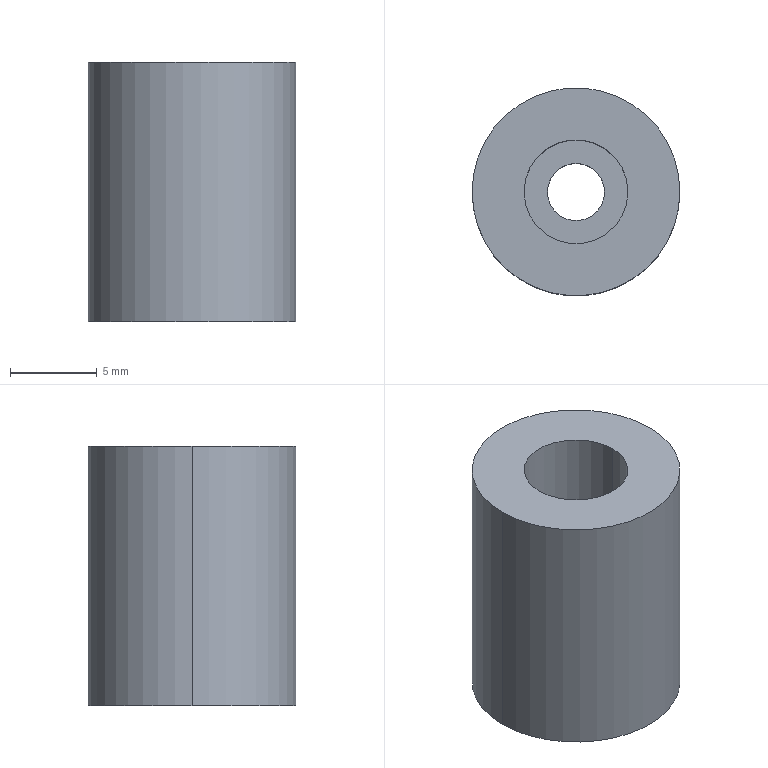Part | SolidWorks | features Extrusion 1, HoleWzd 1 | 1 solid | 9 faces | box 12 x 12 x 15 mm | volume 1371 mm3 | cylinder 6 | plane 3 | commonest cylinder face diameters 3.3 x2 6 x2 12 x2
STEP:
#1=CARTESIAN_POINT('',(-3.,0.,5.));
#2=VERTEX_POINT('',#1);
#3=CARTESIAN_POINT('',(3.,0.,5.));
#4=VERTEX_POINT('',#3);
#5=CARTESIAN_POINT('',(0.,0.,5.));
#6=DIRECTION('',(0.,0.,1.));
#7=DIRECTION('',(1.,0.,0.));
#8=AXIS2_PLACEMENT_3D('',#5,#6,#7);
#9=CIRCLE('',#8,3.);
#10=EDGE_CURVE('',#2,#4,#9,.T.);
#11=ORIENTED_EDGE('',*,*,#10,.F.);
#12=CARTESIAN_POINT('',(-3.,0.,15.));
#13=VERTEX_POINT('',#12);
#14=CARTESIAN_POINT('',(-3.,0.,15.));
#15=DIRECTION('',(0.,0.,1.));
#16=VECTOR('',#15,1000.);
#17=LINE('',#14,#16);
#18=EDGE_CURVE('',#2,#13,#17,.T.);
#19=ORIENTED_EDGE('',*,*,#18,.T.);
#20=CARTESIAN_POINT('',(3.,0.,15.));
#21=VERTEX_POINT('',#20);
#22=CARTESIAN_POINT('',(0.,0.,15.));
#23=DIRECTION('',(0.,0.,1.));
#24=DIRECTION('',(1.,0.,0.));
#25=AXIS2_PLACEMENT_3D('',#22,#23,#24);
#26=CIRCLE('',#25,3.);
#27=EDGE_CURVE('',#13,#21,#26,.T.);
#28=ORIENTED_EDGE('',*,*,#27,.T.);
#29=CARTESIAN_POINT('',(3.,0.,15.));
#30=DIRECTION('',(0.,0.,1.));
#31=VECTOR('',#30,1000.);
#32=LINE('',#29,#31);
#33=EDGE_CURVE('',#4,#21,#32,.T.);
#34=ORIENTED_EDGE('',*,*,#33,.F.);
#35=EDGE_LOOP('',(#11,#19,#28,#34));
#36=FACE_OUTER_BOUND('',#35,.T.);
#37=CARTESIAN_POINT('',(0.,0.,15.));
#38=DIRECTION('',(0.,0.,1.));
#39=DIRECTION('',(1.,0.,0.));
#40=AXIS2_PLACEMENT_3D('',#37,#38,#39);
#41=CYLINDRICAL_SURFACE('',#40,3.);
#42=ADVANCED_FACE('',(#36),#41,.F.);
#43=CARTESIAN_POINT('',(-1.65,0.,0.));
#44=VERTEX_POINT('',#43);
#45=CARTESIAN_POINT('',(1.65,0.,0.));
#46=VERTEX_POINT('',#45);
#47=CARTESIAN_POINT('',(0.,0.,0.));
#48=DIRECTION('',(0.,0.,1.));
#49=DIRECTION('',(1.,0.,0.));
#50=AXIS2_PLACEMENT_3D('',#47,#48,#49);
#51=CIRCLE('',#50,1.65);
#52=EDGE_CURVE('',#44,#46,#51,.T.);
#53=ORIENTED_EDGE('',*,*,#52,.F.);
#54=CARTESIAN_POINT('',(-1.65,0.,5.));
#55=VERTEX_POINT('',#54);
#56=CARTESIAN_POINT('',(-1.65,0.,15.));
#57=DIRECTION('',(0.,0.,1.));
#58=VECTOR('',#57,1000.);
#59=LINE('',#56,#58);
#60=EDGE_CURVE('',#44,#55,#59,.T.);
#61=ORIENTED_EDGE('',*,*,#60,.T.);
#62=CARTESIAN_POINT('',(1.65,0.,5.));
#63=VERTEX_POINT('',#62);
#64=CARTESIAN_POINT('',(0.,0.,5.));
#65=DIRECTION('',(0.,0.,1.));
#66=DIRECTION('',(1.,0.,0.));
#67=AXIS2_PLACEMENT_3D('',#64,#65,#66);
#68=CIRCLE('',#67,1.65);
#69=EDGE_CURVE('',#55,#63,#68,.T.);
#70=ORIENTED_EDGE('',*,*,#69,.T.);
#71=CARTESIAN_POINT('',(1.65,0.,15.));
#72=DIRECTION('',(0.,0.,1.));
#73=VECTOR('',#72,1000.);
#74=LINE('',#71,#73);
#75=EDGE_CURVE('',#46,#63,#74,.T.);
#76=ORIENTED_EDGE('',*,*,#75,.F.);
#77=EDGE_LOOP('',(#53,#61,#70,#76));
#78=FACE_OUTER_BOUND('',#77,.T.);
#79=CARTESIAN_POINT('',(0.,0.,15.));
#80=DIRECTION('',(0.,0.,1.));
#81=DIRECTION('',(1.,0.,0.));
#82=AXIS2_PLACEMENT_3D('',#79,#80,#81);
#83=CYLINDRICAL_SURFACE('',#82,1.65);
#84=ADVANCED_FACE('',(#78),#83,.F.);
#85=CARTESIAN_POINT('',(6.,0.,15.));
#86=VERTEX_POINT('',#85);
#87=CARTESIAN_POINT('',(-6.,0.,15.));
#88=VERTEX_POINT('',#87);
#89=CARTESIAN_POINT('',(0.,0.,15.));
#90=DIRECTION('',(0.,0.,1.));
#91=DIRECTION('',(1.,0.,0.));
#92=AXIS2_PLACEMENT_3D('',#89,#90,#91);
#93=CIRCLE('',#92,6.);
#94=EDGE_CURVE('',#86,#88,#93,.T.);
#95=ORIENTED_EDGE('',*,*,#94,.F.);
#96=CARTESIAN_POINT('',(6.,0.,0.));
#97=VERTEX_POINT('',#96);
#98=CARTESIAN_POINT('',(6.,0.,15.));
#99=DIRECTION('',(0.,0.,-1.));
#100=VECTOR('',#99,1000.);
#101=LINE('',#98,#100);
#102=EDGE_CURVE('',#86,#97,#101,.T.);
#103=ORIENTED_EDGE('',*,*,#102,.T.);
#104=CARTESIAN_POINT('',(-6.,0.,0.));
#105=VERTEX_POINT('',#104);
#106=CARTESIAN_POINT('',(0.,0.,0.));
#107=DIRECTION('',(0.,0.,1.));
#108=DIRECTION('',(1.,0.,0.));
#109=AXIS2_PLACEMENT_3D('',#106,#107,#108);
#110=CIRCLE('',#109,6.);
#111=EDGE_CURVE('',#97,#105,#110,.T.);
#112=ORIENTED_EDGE('',*,*,#111,.T.);
#113=CARTESIAN_POINT('',(-6.,0.,15.));
#114=DIRECTION('',(0.,0.,-1.));
#115=VECTOR('',#114,1000.);
#116=LINE('',#113,#115);
#117=EDGE_CURVE('',#88,#105,#116,.T.);
#118=ORIENTED_EDGE('',*,*,#117,.F.);
#119=EDGE_LOOP('',(#95,#103,#112,#118));
#120=FACE_OUTER_BOUND('',#119,.T.);
#121=CARTESIAN_POINT('',(0.,0.,15.));
#122=DIRECTION('',(0.,0.,-1.));
#123=DIRECTION('',(-1.,0.,0.));
#124=AXIS2_PLACEMENT_3D('',#121,#122,#123);
#125=CYLINDRICAL_SURFACE('',#124,6.);
#126=ADVANCED_FACE('',(#120),#125,.T.);
#127=ORIENTED_EDGE('',*,*,#102,.F.);
#128=CARTESIAN_POINT('',(0.,0.,15.));
#129=DIRECTION('',(0.,0.,1.));
#130=DIRECTION('',(1.,0.,0.));
#131=AXIS2_PLACEMENT_3D('',#128,#129,#130);
#132=CIRCLE('',#131,6.);
#133=EDGE_CURVE('',#88,#86,#132,.T.);
#134=ORIENTED_EDGE('',*,*,#133,.F.);
#135=ORIENTED_EDGE('',*,*,#117,.T.);
#136=CARTESIAN_POINT('',(0.,0.,0.));
#137=DIRECTION('',(0.,0.,1.));
#138=DIRECTION('',(1.,0.,0.));
#139=AXIS2_PLACEMENT_3D('',#136,#137,#138);
#140=CIRCLE('',#139,6.);
#141=EDGE_CURVE('',#105,#97,#140,.T.);
#142=ORIENTED_EDGE('',*,*,#141,.T.);
#143=EDGE_LOOP('',(#127,#134,#135,#142));
#144=FACE_OUTER_BOUND('',#143,.T.);
#145=CARTESIAN_POINT('',(0.,0.,15.));
#146=DIRECTION('',(0.,0.,-1.));
#147=DIRECTION('',(-1.,0.,0.));
#148=AXIS2_PLACEMENT_3D('',#145,#146,#147);
#149=CYLINDRICAL_SURFACE('',#148,6.);
#150=ADVANCED_FACE('',(#144),#149,.T.);
#151=CARTESIAN_POINT('',(0.,0.,15.));
#152=DIRECTION('',(0.,0.,1.));
#153=DIRECTION('',(1.,0.,0.));
#154=AXIS2_PLACEMENT_3D('',#151,#152,#153);
#155=CIRCLE('',#154,3.);
#156=EDGE_CURVE('',#21,#13,#155,.T.);
#157=ORIENTED_EDGE('',*,*,#156,.F.);
#158=ORIENTED_EDGE('',*,*,#27,.F.);
#159=EDGE_LOOP('',(#157,#158));
#160=FACE_BOUND('',#159,.T.);
#161=ORIENTED_EDGE('',*,*,#133,.T.);
#162=ORIENTED_EDGE('',*,*,#94,.T.);
#163=EDGE_LOOP('',(#161,#162));
#164=FACE_OUTER_BOUND('',#163,.T.);
#165=CARTESIAN_POINT('',(0.,0.,15.));
#166=DIRECTION('',(0.,0.,1.));
#167=DIRECTION('',(1.,0.,0.));
#168=AXIS2_PLACEMENT_3D('',#165,#166,#167);
#169=PLANE('',#168);
#170=ADVANCED_FACE('',(#160,#164),#169,.T.);
#171=CARTESIAN_POINT('',(0.,0.,0.));
#172=DIRECTION('',(0.,0.,1.));
#173=DIRECTION('',(1.,0.,0.));
#174=AXIS2_PLACEMENT_3D('',#171,#172,#173);
#175=CIRCLE('',#174,1.65);
#176=EDGE_CURVE('',#46,#44,#175,.T.);
#177=ORIENTED_EDGE('',*,*,#176,.T.);
#178=ORIENTED_EDGE('',*,*,#52,.T.);
#179=EDGE_LOOP('',(#177,#178));
#180=FACE_BOUND('',#179,.T.);
#181=ORIENTED_EDGE('',*,*,#141,.F.);
#182=ORIENTED_EDGE('',*,*,#111,.F.);
#183=EDGE_LOOP('',(#181,#182));
#184=FACE_OUTER_BOUND('',#183,.T.);
#185=CARTESIAN_POINT('',(0.,0.,0.));
#186=DIRECTION('',(0.,0.,1.));
#187=DIRECTION('',(1.,0.,0.));
#188=AXIS2_PLACEMENT_3D('',#185,#186,#187);
#189=PLANE('',#188);
#190=ADVANCED_FACE('',(#180,#184),#189,.F.);
#191=ORIENTED_EDGE('',*,*,#60,.F.);
#192=ORIENTED_EDGE('',*,*,#176,.F.);
#193=ORIENTED_EDGE('',*,*,#75,.T.);
#194=CARTESIAN_POINT('',(0.,0.,5.));
#195=DIRECTION('',(0.,0.,1.));
#196=DIRECTION('',(1.,0.,0.));
#197=AXIS2_PLACEMENT_3D('',#194,#195,#196);
#198=CIRCLE('',#197,1.65);
#199=EDGE_CURVE('',#63,#55,#198,.T.);
#200=ORIENTED_EDGE('',*,*,#199,.T.);
#201=EDGE_LOOP('',(#191,#192,#193,#200));
#202=FACE_OUTER_BOUND('',#201,.T.);
#203=CARTESIAN_POINT('',(0.,0.,15.));
#204=DIRECTION('',(0.,0.,1.));
#205=DIRECTION('',(1.,0.,0.));
#206=AXIS2_PLACEMENT_3D('',#203,#204,#205);
#207=CYLINDRICAL_SURFACE('',#206,1.65);
#208=ADVANCED_FACE('',(#202),#207,.F.);
#209=ORIENTED_EDGE('',*,*,#199,.F.);
#210=ORIENTED_EDGE('',*,*,#69,.F.);
#211=EDGE_LOOP('',(#209,#210));
#212=FACE_BOUND('',#211,.T.);
#213=CARTESIAN_POINT('',(0.,0.,5.));
#214=DIRECTION('',(0.,0.,1.));
#215=DIRECTION('',(1.,0.,0.));
#216=AXIS2_PLACEMENT_3D('',#213,#214,#215);
#217=CIRCLE('',#216,3.);
#218=EDGE_CURVE('',#4,#2,#217,.T.);
#219=ORIENTED_EDGE('',*,*,#218,.T.);
#220=ORIENTED_EDGE('',*,*,#10,.T.);
#221=EDGE_LOOP('',(#219,#220));
#222=FACE_OUTER_BOUND('',#221,.T.);
#223=CARTESIAN_POINT('',(1.65,0.,5.));
#224=DIRECTION('',(0.,0.,-1.));
#225=DIRECTION('',(-1.,0.,0.));
#226=AXIS2_PLACEMENT_3D('',#223,#224,#225);
#227=PLANE('',#226);
#228=ADVANCED_FACE('',(#212,#222),#227,.F.);
#229=ORIENTED_EDGE('',*,*,#18,.F.);
#230=ORIENTED_EDGE('',*,*,#218,.F.);
#231=ORIENTED_EDGE('',*,*,#33,.T.);
#232=ORIENTED_EDGE('',*,*,#156,.T.);
#233=EDGE_LOOP('',(#229,#230,#231,#232));
#234=FACE_OUTER_BOUND('',#233,.T.);
#235=CARTESIAN_POINT('',(0.,0.,15.));
#236=DIRECTION('',(0.,0.,1.));
#237=DIRECTION('',(1.,0.,0.));
#238=AXIS2_PLACEMENT_3D('',#235,#236,#237);
#239=CYLINDRICAL_SURFACE('',#238,3.);
#240=ADVANCED_FACE('',(#234),#239,.F.);
#241=CLOSED_SHELL('',(#42,#84,#126,#150,#170,#190,#208,#228,#240));
#242=MANIFOLD_SOLID_BREP('',#241);
#243=CARTESIAN_POINT('',(0.,0.,0.));
#244=DIRECTION('',(0.,0.,1.));
#245=DIRECTION('',(1.,0.,0.));
#246=AXIS2_PLACEMENT_3D('',#243,#244,#245);
#247=(LENGTH_UNIT()NAMED_UNIT(*)SI_UNIT(.MILLI.,.METRE.));
#248=UNCERTAINTY_MEASURE_WITH_UNIT(LENGTH_MEASURE(0.00001),#247,'','');
#249=(NAMED_UNIT(*)PLANE_ANGLE_UNIT()SI_UNIT($,.RADIAN.));
#250=(NAMED_UNIT(*)SI_UNIT($,.STERADIAN.)SOLID_ANGLE_UNIT());
#251=(GEOMETRIC_REPRESENTATION_CONTEXT(3)GLOBAL_UNCERTAINTY_ASSIGNED_CONTEXT((#248))GLOBAL_UNIT_ASSIGNED_CONTEXT((#247,#249,#250))REPRESENTATION_CONTEXT('',''));
#252=ADVANCED_BREP_SHAPE_REPRESENTATION('',(#242,#246),#251);